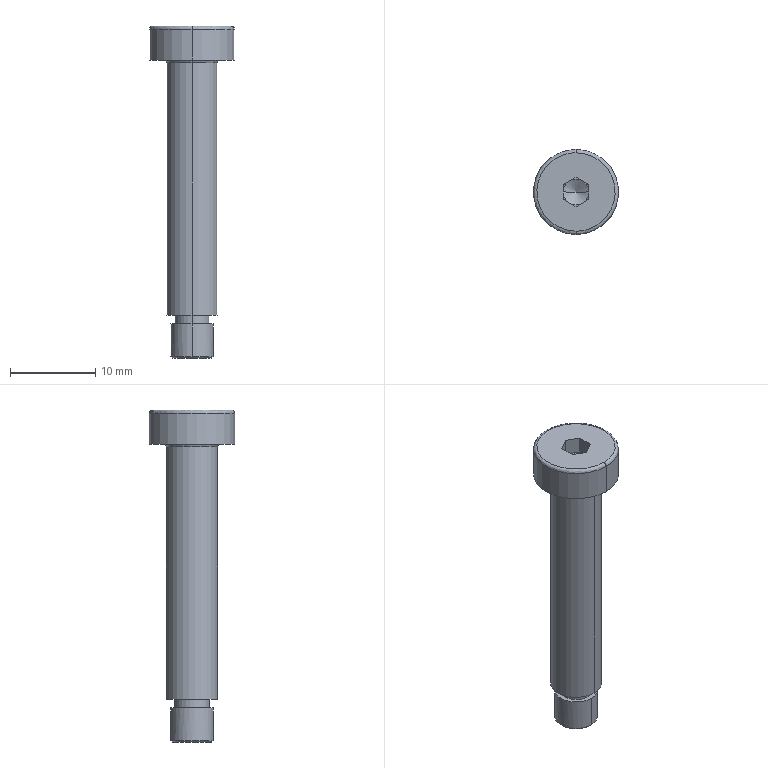Part | STEP file | free-specified tolerance g6 equal-height bolt[HSBGFS6-30-5-5]_HSBGFS6-30-5-5 | 1 solid | 33 faces | box 10 x 10 x 39 mm | volume 1235 mm3 | plane 17 | cylinder 8 | spline 4 | cone 4 | commonest cylinder face diameters 4 x2 5 x2 6 x2 10 x2